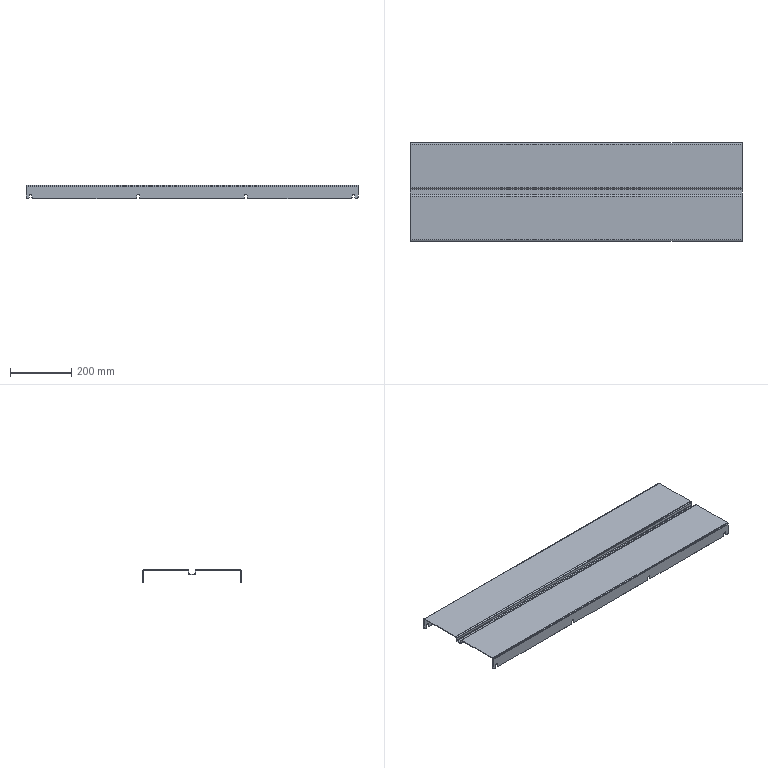Part | STEP file | BELT.PLATE.12.stp | 1 solid | 90 faces | box 1080 x 320 x 43 mm | volume 914400 mm3 | spline 42 | cylinder 28 | plane 20 | commonest cylinder face diameters 10 x12 4 x6 8 x6 9 x4